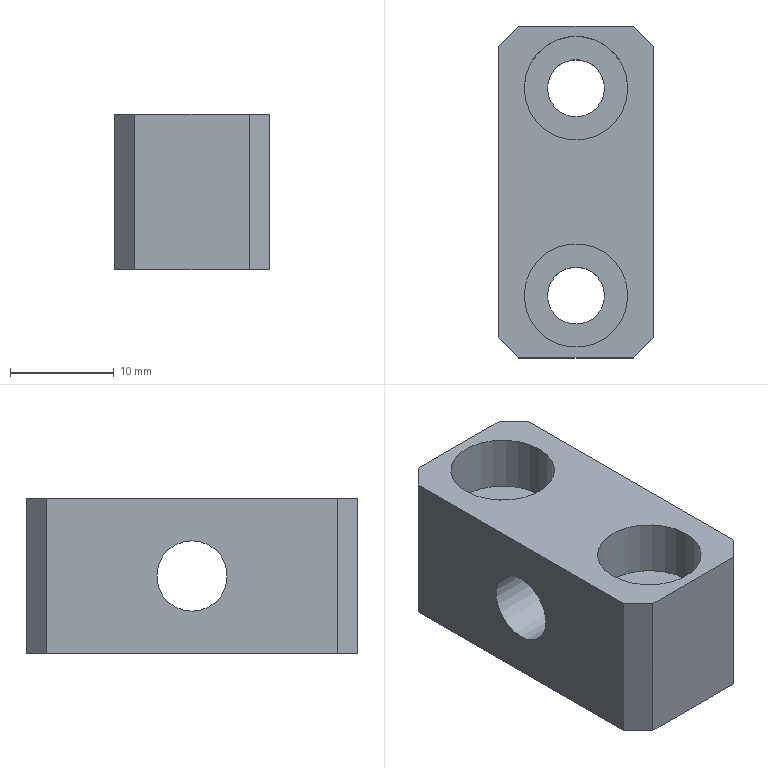Part | NX | 1 solid | 17 faces | box 15 x 32 x 15 mm | volume 5231 mm3 | plane 12 | cylinder 5 | commonest cylinder face diameters 5.5 x2 10 x2 6.8 x1
STEP:
#1=CARTESIAN_POINT('',(7.5,0.,4.1));
#2=VERTEX_POINT('',#1);
#3=CARTESIAN_POINT('',(7.5,0.,7.5));
#4=DIRECTION('',(1.,0.,0.));
#5=DIRECTION('',(0.,0.,-1.));
#6=AXIS2_PLACEMENT_3D('',#3,#4,#5);
#7=CIRCLE('',#6,3.4);
#8=EDGE_CURVE('',#2,#2,#7,.T.);
#9=ORIENTED_EDGE('',*,*,#8,.F.);
#10=EDGE_LOOP('',(#9));
#11=FACE_BOUND('',#10,.T.);
#12=CARTESIAN_POINT('',(7.5,-14.,15.));
#13=VERTEX_POINT('',#12);
#14=CARTESIAN_POINT('',(7.5,14.,15.));
#15=VERTEX_POINT('',#14);
#16=CARTESIAN_POINT('',(7.5,-16.,15.));
#17=DIRECTION('',(0.,1.,0.));
#18=VECTOR('',#17,1000.);
#19=LINE('',#16,#18);
#20=EDGE_CURVE('',#13,#15,#19,.T.);
#21=ORIENTED_EDGE('',*,*,#20,.F.);
#22=CARTESIAN_POINT('',(7.5,-14.,0.));
#23=VERTEX_POINT('',#22);
#24=CARTESIAN_POINT('',(7.5,-14.,15.));
#25=DIRECTION('',(0.,0.,-1.));
#26=VECTOR('',#25,1000.);
#27=LINE('',#24,#26);
#28=EDGE_CURVE('',#13,#23,#27,.T.);
#29=ORIENTED_EDGE('',*,*,#28,.T.);
#30=CARTESIAN_POINT('',(7.5,14.,0.));
#31=VERTEX_POINT('',#30);
#32=CARTESIAN_POINT('',(7.5,-16.,0.));
#33=DIRECTION('',(0.,1.,0.));
#34=VECTOR('',#33,1000.);
#35=LINE('',#32,#34);
#36=EDGE_CURVE('',#23,#31,#35,.T.);
#37=ORIENTED_EDGE('',*,*,#36,.T.);
#38=CARTESIAN_POINT('',(7.5,14.,15.));
#39=DIRECTION('',(0.,0.,1.));
#40=VECTOR('',#39,1000.);
#41=LINE('',#38,#40);
#42=EDGE_CURVE('',#31,#15,#41,.T.);
#43=ORIENTED_EDGE('',*,*,#42,.T.);
#44=EDGE_LOOP('',(#21,#29,#37,#43));
#45=FACE_BOUND('',#44,.T.);
#46=CARTESIAN_POINT('',(7.5,-16.,15.));
#47=DIRECTION('',(-1.,0.,0.));
#48=DIRECTION('',(0.,0.,1.));
#49=AXIS2_PLACEMENT_3D('',#46,#47,#48);
#50=PLANE('',#49);
#51=ADVANCED_FACE('',(#11,#45),#50,.F.);
#52=CARTESIAN_POINT('',(5.5,16.,0.));
#53=VERTEX_POINT('',#52);
#54=CARTESIAN_POINT('',(-5.5,16.,0.));
#55=VERTEX_POINT('',#54);
#56=CARTESIAN_POINT('',(-7.5,16.,0.));
#57=DIRECTION('',(-1.,0.,0.));
#58=VECTOR('',#57,1000.);
#59=LINE('',#56,#58);
#60=EDGE_CURVE('',#53,#55,#59,.T.);
#61=ORIENTED_EDGE('',*,*,#60,.T.);
#62=CARTESIAN_POINT('',(-5.5,16.,15.));
#63=VERTEX_POINT('',#62);
#64=CARTESIAN_POINT('',(-5.5,16.,15.));
#65=DIRECTION('',(0.,0.,1.));
#66=VECTOR('',#65,1000.);
#67=LINE('',#64,#66);
#68=EDGE_CURVE('',#55,#63,#67,.T.);
#69=ORIENTED_EDGE('',*,*,#68,.T.);
#70=CARTESIAN_POINT('',(5.5,16.,15.));
#71=VERTEX_POINT('',#70);
#72=CARTESIAN_POINT('',(-7.5,16.,15.));
#73=DIRECTION('',(-1.,0.,0.));
#74=VECTOR('',#73,1000.);
#75=LINE('',#72,#74);
#76=EDGE_CURVE('',#71,#63,#75,.T.);
#77=ORIENTED_EDGE('',*,*,#76,.F.);
#78=CARTESIAN_POINT('',(5.5,16.,15.));
#79=DIRECTION('',(0.,0.,-1.));
#80=VECTOR('',#79,1000.);
#81=LINE('',#78,#80);
#82=EDGE_CURVE('',#71,#53,#81,.T.);
#83=ORIENTED_EDGE('',*,*,#82,.T.);
#84=EDGE_LOOP('',(#61,#69,#77,#83));
#85=FACE_BOUND('',#84,.T.);
#86=CARTESIAN_POINT('',(-7.5,16.,15.));
#87=DIRECTION('',(0.,-1.,0.));
#88=DIRECTION('',(0.,0.,-1.));
#89=AXIS2_PLACEMENT_3D('',#86,#87,#88);
#90=PLANE('',#89);
#91=ADVANCED_FACE('',(#85),#90,.F.);
#92=CARTESIAN_POINT('',(-7.5,0.,4.1));
#93=VERTEX_POINT('',#92);
#94=CARTESIAN_POINT('',(-7.5,0.,7.5));
#95=DIRECTION('',(1.,0.,0.));
#96=DIRECTION('',(0.,0.,-1.));
#97=AXIS2_PLACEMENT_3D('',#94,#95,#96);
#98=CIRCLE('',#97,3.4);
#99=EDGE_CURVE('',#93,#93,#98,.T.);
#100=ORIENTED_EDGE('',*,*,#99,.T.);
#101=EDGE_LOOP('',(#100));
#102=FACE_BOUND('',#101,.T.);
#103=CARTESIAN_POINT('',(-7.5,14.,0.));
#104=VERTEX_POINT('',#103);
#105=CARTESIAN_POINT('',(-7.5,-14.,0.));
#106=VERTEX_POINT('',#105);
#107=CARTESIAN_POINT('',(-7.5,-16.,0.));
#108=DIRECTION('',(0.,-1.,0.));
#109=VECTOR('',#108,1000.);
#110=LINE('',#107,#109);
#111=EDGE_CURVE('',#104,#106,#110,.T.);
#112=ORIENTED_EDGE('',*,*,#111,.T.);
#113=CARTESIAN_POINT('',(-7.5,-14.,15.));
#114=VERTEX_POINT('',#113);
#115=CARTESIAN_POINT('',(-7.5,-14.,15.));
#116=DIRECTION('',(0.,0.,1.));
#117=VECTOR('',#116,1000.);
#118=LINE('',#115,#117);
#119=EDGE_CURVE('',#106,#114,#118,.T.);
#120=ORIENTED_EDGE('',*,*,#119,.T.);
#121=CARTESIAN_POINT('',(-7.5,14.,15.));
#122=VERTEX_POINT('',#121);
#123=CARTESIAN_POINT('',(-7.5,-16.,15.));
#124=DIRECTION('',(0.,-1.,0.));
#125=VECTOR('',#124,1000.);
#126=LINE('',#123,#125);
#127=EDGE_CURVE('',#122,#114,#126,.T.);
#128=ORIENTED_EDGE('',*,*,#127,.F.);
#129=CARTESIAN_POINT('',(-7.5,14.,15.));
#130=DIRECTION('',(0.,0.,-1.));
#131=VECTOR('',#130,1000.);
#132=LINE('',#129,#131);
#133=EDGE_CURVE('',#122,#104,#132,.T.);
#134=ORIENTED_EDGE('',*,*,#133,.T.);
#135=EDGE_LOOP('',(#112,#120,#128,#134));
#136=FACE_BOUND('',#135,.T.);
#137=CARTESIAN_POINT('',(-7.5,-16.,15.));
#138=DIRECTION('',(1.,0.,0.));
#139=DIRECTION('',(0.,0.,-1.));
#140=AXIS2_PLACEMENT_3D('',#137,#138,#139);
#141=PLANE('',#140);
#142=ADVANCED_FACE('',(#102,#136),#141,.F.);
#143=CARTESIAN_POINT('',(-5.5,-16.,15.));
#144=VERTEX_POINT('',#143);
#145=CARTESIAN_POINT('',(5.5,-16.,15.));
#146=VERTEX_POINT('',#145);
#147=CARTESIAN_POINT('',(-7.5,-16.,15.));
#148=DIRECTION('',(1.,0.,0.));
#149=VECTOR('',#148,1000.);
#150=LINE('',#147,#149);
#151=EDGE_CURVE('',#144,#146,#150,.T.);
#152=ORIENTED_EDGE('',*,*,#151,.F.);
#153=CARTESIAN_POINT('',(-5.5,-16.,0.));
#154=VERTEX_POINT('',#153);
#155=CARTESIAN_POINT('',(-5.5,-16.,15.));
#156=DIRECTION('',(0.,0.,-1.));
#157=VECTOR('',#156,1000.);
#158=LINE('',#155,#157);
#159=EDGE_CURVE('',#144,#154,#158,.T.);
#160=ORIENTED_EDGE('',*,*,#159,.T.);
#161=CARTESIAN_POINT('',(5.5,-16.,0.));
#162=VERTEX_POINT('',#161);
#163=CARTESIAN_POINT('',(-7.5,-16.,0.));
#164=DIRECTION('',(1.,0.,0.));
#165=VECTOR('',#164,1000.);
#166=LINE('',#163,#165);
#167=EDGE_CURVE('',#154,#162,#166,.T.);
#168=ORIENTED_EDGE('',*,*,#167,.T.);
#169=CARTESIAN_POINT('',(5.5,-16.,15.));
#170=DIRECTION('',(0.,0.,1.));
#171=VECTOR('',#170,1000.);
#172=LINE('',#169,#171);
#173=EDGE_CURVE('',#162,#146,#172,.T.);
#174=ORIENTED_EDGE('',*,*,#173,.T.);
#175=EDGE_LOOP('',(#152,#160,#168,#174));
#176=FACE_BOUND('',#175,.T.);
#177=CARTESIAN_POINT('',(-7.5,-16.,15.));
#178=DIRECTION('',(0.,1.,0.));
#179=DIRECTION('',(0.,0.,1.));
#180=AXIS2_PLACEMENT_3D('',#177,#178,#179);
#181=PLANE('',#180);
#182=ADVANCED_FACE('',(#176),#181,.F.);
#183=CARTESIAN_POINT('',(5.,10.,15.));
#184=VERTEX_POINT('',#183);
#185=CARTESIAN_POINT('',(0.,10.,15.));
#186=DIRECTION('',(0.,0.,1.));
#187=DIRECTION('',(1.,0.,0.));
#188=AXIS2_PLACEMENT_3D('',#185,#186,#187);
#189=CIRCLE('',#188,5.);
#190=EDGE_CURVE('',#184,#184,#189,.T.);
#191=ORIENTED_EDGE('',*,*,#190,.F.);
#192=EDGE_LOOP('',(#191));
#193=FACE_BOUND('',#192,.T.);
#194=CARTESIAN_POINT('',(5.,-10.,15.));
#195=VERTEX_POINT('',#194);
#196=CARTESIAN_POINT('',(0.,-10.,15.));
#197=DIRECTION('',(0.,0.,1.));
#198=DIRECTION('',(1.,0.,0.));
#199=AXIS2_PLACEMENT_3D('',#196,#197,#198);
#200=CIRCLE('',#199,5.);
#201=EDGE_CURVE('',#195,#195,#200,.T.);
#202=ORIENTED_EDGE('',*,*,#201,.F.);
#203=EDGE_LOOP('',(#202));
#204=FACE_BOUND('',#203,.T.);
#205=ORIENTED_EDGE('',*,*,#127,.T.);
#206=CARTESIAN_POINT('',(-5.5,-16.,15.));
#207=DIRECTION('',(-0.7071,0.7071,0.));
#208=VECTOR('',#207,1000.);
#209=LINE('',#206,#208);
#210=EDGE_CURVE('',#114,#144,#209,.F.);
#211=ORIENTED_EDGE('',*,*,#210,.T.);
#212=ORIENTED_EDGE('',*,*,#151,.T.);
#213=CARTESIAN_POINT('',(7.5,-14.,15.));
#214=DIRECTION('',(-0.7071,-0.7071,0.));
#215=VECTOR('',#214,1000.);
#216=LINE('',#213,#215);
#217=EDGE_CURVE('',#146,#13,#216,.F.);
#218=ORIENTED_EDGE('',*,*,#217,.T.);
#219=ORIENTED_EDGE('',*,*,#20,.T.);
#220=CARTESIAN_POINT('',(5.5,16.,15.));
#221=DIRECTION('',(0.7071,-0.7071,0.));
#222=VECTOR('',#221,1000.);
#223=LINE('',#220,#222);
#224=EDGE_CURVE('',#15,#71,#223,.F.);
#225=ORIENTED_EDGE('',*,*,#224,.T.);
#226=ORIENTED_EDGE('',*,*,#76,.T.);
#227=CARTESIAN_POINT('',(-7.5,14.,15.));
#228=DIRECTION('',(0.7071,0.7071,0.));
#229=VECTOR('',#228,1000.);
#230=LINE('',#227,#229);
#231=EDGE_CURVE('',#63,#122,#230,.F.);
#232=ORIENTED_EDGE('',*,*,#231,.T.);
#233=EDGE_LOOP('',(#205,#211,#212,#218,#219,#225,#226,#232));
#234=FACE_BOUND('',#233,.T.);
#235=CARTESIAN_POINT('',(0.,0.,15.));
#236=DIRECTION('',(0.,0.,-1.));
#237=DIRECTION('',(-1.,0.,0.));
#238=AXIS2_PLACEMENT_3D('',#235,#236,#237);
#239=PLANE('',#238);
#240=ADVANCED_FACE('',(#193,#204,#234),#239,.F.);
#241=CARTESIAN_POINT('',(2.75,10.,0.));
#242=VERTEX_POINT('',#241);
#243=CARTESIAN_POINT('',(0.,10.,0.));
#244=DIRECTION('',(0.,0.,1.));
#245=DIRECTION('',(1.,0.,0.));
#246=AXIS2_PLACEMENT_3D('',#243,#244,#245);
#247=CIRCLE('',#246,2.75);
#248=EDGE_CURVE('',#242,#242,#247,.T.);
#249=ORIENTED_EDGE('',*,*,#248,.T.);
#250=EDGE_LOOP('',(#249));
#251=FACE_BOUND('',#250,.T.);
#252=CARTESIAN_POINT('',(2.75,-10.,0.));
#253=VERTEX_POINT('',#252);
#254=CARTESIAN_POINT('',(0.,-10.,0.));
#255=DIRECTION('',(0.,0.,1.));
#256=DIRECTION('',(1.,0.,0.));
#257=AXIS2_PLACEMENT_3D('',#254,#255,#256);
#258=CIRCLE('',#257,2.75);
#259=EDGE_CURVE('',#253,#253,#258,.T.);
#260=ORIENTED_EDGE('',*,*,#259,.T.);
#261=EDGE_LOOP('',(#260));
#262=FACE_BOUND('',#261,.T.);
#263=ORIENTED_EDGE('',*,*,#167,.F.);
#264=CARTESIAN_POINT('',(-10.75,-10.75,0.));
#265=DIRECTION('',(0.7071,-0.7071,0.));
#266=VECTOR('',#265,1000.);
#267=LINE('',#264,#266);
#268=EDGE_CURVE('',#154,#106,#267,.F.);
#269=ORIENTED_EDGE('',*,*,#268,.T.);
#270=ORIENTED_EDGE('',*,*,#111,.F.);
#271=CARTESIAN_POINT('',(-10.75,10.75,0.));
#272=DIRECTION('',(-0.7071,-0.7071,0.));
#273=VECTOR('',#272,1000.);
#274=LINE('',#271,#273);
#275=EDGE_CURVE('',#104,#55,#274,.F.);
#276=ORIENTED_EDGE('',*,*,#275,.T.);
#277=ORIENTED_EDGE('',*,*,#60,.F.);
#278=CARTESIAN_POINT('',(10.75,10.75,0.));
#279=DIRECTION('',(-0.7071,0.7071,0.));
#280=VECTOR('',#279,1000.);
#281=LINE('',#278,#280);
#282=EDGE_CURVE('',#53,#31,#281,.F.);
#283=ORIENTED_EDGE('',*,*,#282,.T.);
#284=ORIENTED_EDGE('',*,*,#36,.F.);
#285=CARTESIAN_POINT('',(10.75,-10.75,0.));
#286=DIRECTION('',(0.7071,0.7071,0.));
#287=VECTOR('',#286,1000.);
#288=LINE('',#285,#287);
#289=EDGE_CURVE('',#23,#162,#288,.F.);
#290=ORIENTED_EDGE('',*,*,#289,.T.);
#291=EDGE_LOOP('',(#263,#269,#270,#276,#277,#283,#284,#290));
#292=FACE_BOUND('',#291,.T.);
#293=CARTESIAN_POINT('',(0.,0.,0.));
#294=DIRECTION('',(0.,0.,-1.));
#295=DIRECTION('',(-1.,0.,0.));
#296=AXIS2_PLACEMENT_3D('',#293,#294,#295);
#297=PLANE('',#296);
#298=ADVANCED_FACE('',(#251,#262,#292),#297,.T.);
#299=ORIENTED_EDGE('',*,*,#210,.F.);
#300=ORIENTED_EDGE('',*,*,#119,.F.);
#301=ORIENTED_EDGE('',*,*,#268,.F.);
#302=ORIENTED_EDGE('',*,*,#159,.F.);
#303=EDGE_LOOP('',(#299,#300,#301,#302));
#304=FACE_BOUND('',#303,.T.);
#305=CARTESIAN_POINT('',(-5.5,-16.,15.));
#306=DIRECTION('',(0.7071,0.7071,0.));
#307=DIRECTION('',(0.,0.,-1.));
#308=AXIS2_PLACEMENT_3D('',#305,#306,#307);
#309=PLANE('',#308);
#310=ADVANCED_FACE('',(#304),#309,.F.);
#311=ORIENTED_EDGE('',*,*,#217,.F.);
#312=ORIENTED_EDGE('',*,*,#173,.F.);
#313=ORIENTED_EDGE('',*,*,#289,.F.);
#314=ORIENTED_EDGE('',*,*,#28,.F.);
#315=EDGE_LOOP('',(#311,#312,#313,#314));
#316=FACE_BOUND('',#315,.T.);
#317=CARTESIAN_POINT('',(7.5,-14.,15.));
#318=DIRECTION('',(-0.7071,0.7071,0.));
#319=DIRECTION('',(0.,0.,-1.));
#320=AXIS2_PLACEMENT_3D('',#317,#318,#319);
#321=PLANE('',#320);
#322=ADVANCED_FACE('',(#316),#321,.F.);
#323=ORIENTED_EDGE('',*,*,#231,.F.);
#324=ORIENTED_EDGE('',*,*,#68,.F.);
#325=ORIENTED_EDGE('',*,*,#275,.F.);
#326=ORIENTED_EDGE('',*,*,#133,.F.);
#327=EDGE_LOOP('',(#323,#324,#325,#326));
#328=FACE_BOUND('',#327,.T.);
#329=CARTESIAN_POINT('',(-7.5,14.,15.));
#330=DIRECTION('',(0.7071,-0.7071,0.));
#331=DIRECTION('',(0.,0.,-1.));
#332=AXIS2_PLACEMENT_3D('',#329,#330,#331);
#333=PLANE('',#332);
#334=ADVANCED_FACE('',(#328),#333,.F.);
#335=ORIENTED_EDGE('',*,*,#224,.F.);
#336=ORIENTED_EDGE('',*,*,#42,.F.);
#337=ORIENTED_EDGE('',*,*,#282,.F.);
#338=ORIENTED_EDGE('',*,*,#82,.F.);
#339=EDGE_LOOP('',(#335,#336,#337,#338));
#340=FACE_BOUND('',#339,.T.);
#341=CARTESIAN_POINT('',(5.5,16.,15.));
#342=DIRECTION('',(-0.7071,-0.7071,0.));
#343=DIRECTION('',(0.,0.,-1.));
#344=AXIS2_PLACEMENT_3D('',#341,#342,#343);
#345=PLANE('',#344);
#346=ADVANCED_FACE('',(#340),#345,.F.);
#347=ORIENTED_EDGE('',*,*,#259,.F.);
#348=EDGE_LOOP('',(#347));
#349=FACE_BOUND('',#348,.T.);
#350=CARTESIAN_POINT('',(2.75,-10.,9.6));
#351=VERTEX_POINT('',#350);
#352=CARTESIAN_POINT('',(0.,-10.,9.6));
#353=DIRECTION('',(0.,0.,1.));
#354=DIRECTION('',(1.,0.,0.));
#355=AXIS2_PLACEMENT_3D('',#352,#353,#354);
#356=CIRCLE('',#355,2.75);
#357=EDGE_CURVE('',#351,#351,#356,.T.);
#358=ORIENTED_EDGE('',*,*,#357,.T.);
#359=EDGE_LOOP('',(#358));
#360=FACE_BOUND('',#359,.T.);
#361=CARTESIAN_POINT('',(0.,-10.,15.));
#362=DIRECTION('',(0.,0.,1.));
#363=DIRECTION('',(1.,0.,0.));
#364=AXIS2_PLACEMENT_3D('',#361,#362,#363);
#365=CYLINDRICAL_SURFACE('',#364,2.75);
#366=ADVANCED_FACE('',(#349,#360),#365,.F.);
#367=ORIENTED_EDGE('',*,*,#357,.F.);
#368=EDGE_LOOP('',(#367));
#369=FACE_BOUND('',#368,.T.);
#370=CARTESIAN_POINT('',(5.,-10.,9.6));
#371=VERTEX_POINT('',#370);
#372=CARTESIAN_POINT('',(0.,-10.,9.6));
#373=DIRECTION('',(0.,0.,1.));
#374=DIRECTION('',(1.,0.,0.));
#375=AXIS2_PLACEMENT_3D('',#372,#373,#374);
#376=CIRCLE('',#375,5.);
#377=EDGE_CURVE('',#371,#371,#376,.T.);
#378=ORIENTED_EDGE('',*,*,#377,.T.);
#379=EDGE_LOOP('',(#378));
#380=FACE_BOUND('',#379,.T.);
#381=CARTESIAN_POINT('',(2.75,-10.,9.6));
#382=DIRECTION('',(0.,0.,-1.));
#383=DIRECTION('',(-1.,0.,0.));
#384=AXIS2_PLACEMENT_3D('',#381,#382,#383);
#385=PLANE('',#384);
#386=ADVANCED_FACE('',(#369,#380),#385,.F.);
#387=ORIENTED_EDGE('',*,*,#377,.F.);
#388=EDGE_LOOP('',(#387));
#389=FACE_BOUND('',#388,.T.);
#390=ORIENTED_EDGE('',*,*,#201,.T.);
#391=EDGE_LOOP('',(#390));
#392=FACE_BOUND('',#391,.T.);
#393=CARTESIAN_POINT('',(0.,-10.,15.));
#394=DIRECTION('',(0.,0.,1.));
#395=DIRECTION('',(1.,0.,0.));
#396=AXIS2_PLACEMENT_3D('',#393,#394,#395);
#397=CYLINDRICAL_SURFACE('',#396,5.);
#398=ADVANCED_FACE('',(#389,#392),#397,.F.);
#399=ORIENTED_EDGE('',*,*,#248,.F.);
#400=EDGE_LOOP('',(#399));
#401=FACE_BOUND('',#400,.T.);
#402=CARTESIAN_POINT('',(2.75,10.,9.6));
#403=VERTEX_POINT('',#402);
#404=CARTESIAN_POINT('',(0.,10.,9.6));
#405=DIRECTION('',(0.,0.,1.));
#406=DIRECTION('',(1.,0.,0.));
#407=AXIS2_PLACEMENT_3D('',#404,#405,#406);
#408=CIRCLE('',#407,2.75);
#409=EDGE_CURVE('',#403,#403,#408,.T.);
#410=ORIENTED_EDGE('',*,*,#409,.T.);
#411=EDGE_LOOP('',(#410));
#412=FACE_BOUND('',#411,.T.);
#413=CARTESIAN_POINT('',(0.,10.,15.));
#414=DIRECTION('',(0.,0.,1.));
#415=DIRECTION('',(1.,0.,0.));
#416=AXIS2_PLACEMENT_3D('',#413,#414,#415);
#417=CYLINDRICAL_SURFACE('',#416,2.75);
#418=ADVANCED_FACE('',(#401,#412),#417,.F.);
#419=ORIENTED_EDGE('',*,*,#409,.F.);
#420=EDGE_LOOP('',(#419));
#421=FACE_BOUND('',#420,.T.);
#422=CARTESIAN_POINT('',(5.,10.,9.6));
#423=VERTEX_POINT('',#422);
#424=CARTESIAN_POINT('',(0.,10.,9.6));
#425=DIRECTION('',(0.,0.,1.));
#426=DIRECTION('',(1.,0.,0.));
#427=AXIS2_PLACEMENT_3D('',#424,#425,#426);
#428=CIRCLE('',#427,5.);
#429=EDGE_CURVE('',#423,#423,#428,.T.);
#430=ORIENTED_EDGE('',*,*,#429,.T.);
#431=EDGE_LOOP('',(#430));
#432=FACE_BOUND('',#431,.T.);
#433=CARTESIAN_POINT('',(2.75,10.,9.6));
#434=DIRECTION('',(0.,0.,-1.));
#435=DIRECTION('',(-1.,0.,0.));
#436=AXIS2_PLACEMENT_3D('',#433,#434,#435);
#437=PLANE('',#436);
#438=ADVANCED_FACE('',(#421,#432),#437,.F.);
#439=ORIENTED_EDGE('',*,*,#429,.F.);
#440=EDGE_LOOP('',(#439));
#441=FACE_BOUND('',#440,.T.);
#442=ORIENTED_EDGE('',*,*,#190,.T.);
#443=EDGE_LOOP('',(#442));
#444=FACE_BOUND('',#443,.T.);
#445=CARTESIAN_POINT('',(0.,10.,15.));
#446=DIRECTION('',(0.,0.,1.));
#447=DIRECTION('',(1.,0.,0.));
#448=AXIS2_PLACEMENT_3D('',#445,#446,#447);
#449=CYLINDRICAL_SURFACE('',#448,5.);
#450=ADVANCED_FACE('',(#441,#444),#449,.F.);
#451=ORIENTED_EDGE('',*,*,#99,.F.);
#452=EDGE_LOOP('',(#451));
#453=FACE_BOUND('',#452,.T.);
#454=ORIENTED_EDGE('',*,*,#8,.T.);
#455=EDGE_LOOP('',(#454));
#456=FACE_BOUND('',#455,.T.);
#457=CARTESIAN_POINT('',(7.5,0.,7.5));
#458=DIRECTION('',(1.,0.,0.));
#459=DIRECTION('',(0.,0.,-1.));
#460=AXIS2_PLACEMENT_3D('',#457,#458,#459);
#461=CYLINDRICAL_SURFACE('',#460,3.4);
#462=ADVANCED_FACE('',(#453,#456),#461,.F.);
#463=CLOSED_SHELL('',(#51,#91,#142,#182,#240,#298,#310,#322,#334,#346,#366,#386,#398,#418,#438,#450,#462));
#464=MANIFOLD_SOLID_BREP('',#463);
#465=(LENGTH_UNIT()NAMED_UNIT(*)SI_UNIT(.MILLI.,.METRE.));
#466=UNCERTAINTY_MEASURE_WITH_UNIT(LENGTH_MEASURE(0.00001),#465,'','');
#467=(NAMED_UNIT(*)PLANE_ANGLE_UNIT()SI_UNIT($,.RADIAN.));
#468=(NAMED_UNIT(*)SI_UNIT($,.STERADIAN.)SOLID_ANGLE_UNIT());
#469=(GEOMETRIC_REPRESENTATION_CONTEXT(3)GLOBAL_UNCERTAINTY_ASSIGNED_CONTEXT((#466))GLOBAL_UNIT_ASSIGNED_CONTEXT((#465,#467,#468))REPRESENTATION_CONTEXT('',''));
#470=ADVANCED_BREP_SHAPE_REPRESENTATION('',(#464),#469);